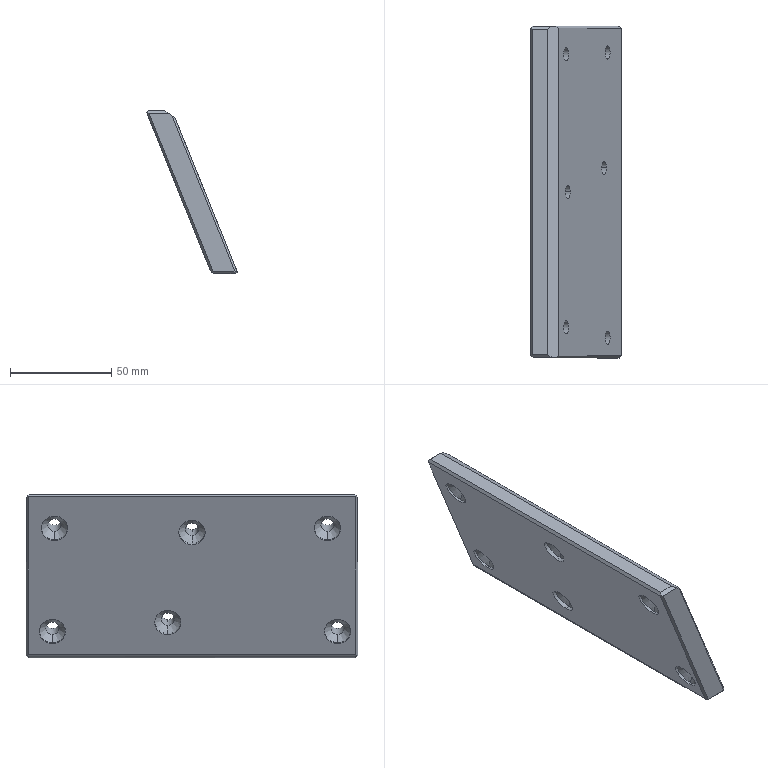Part | Creo | 1 solid | 58 faces | box 44.736 x 164 x 81.01 mm | volume 166179 mm3 | cylinder 25 | plane 21 | cone 12 | commonest cylinder face diameters 6.6 x12 13 x12 6 x1